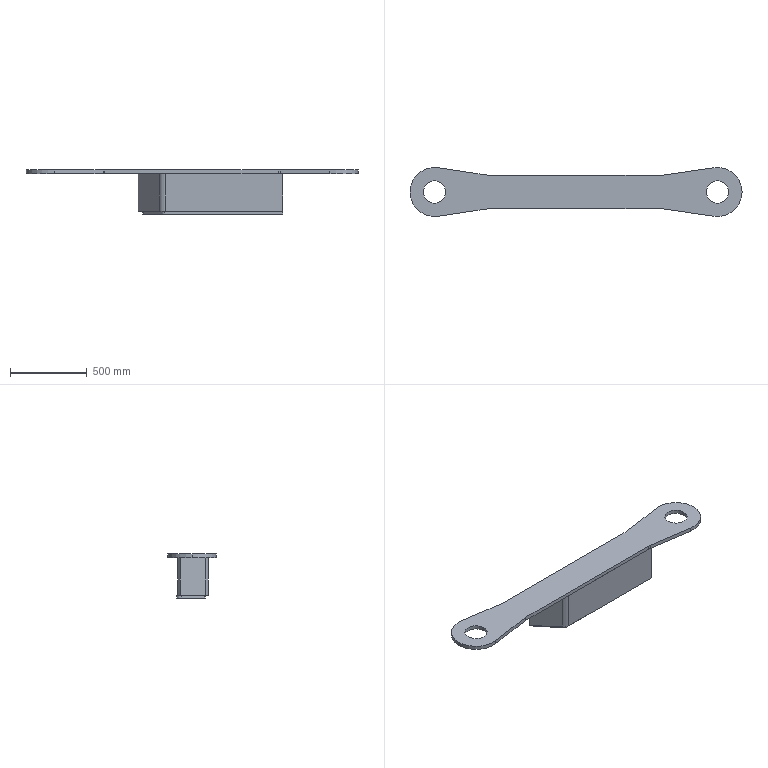Part | NX | features 后连杆左 2 | 1 solid | 48 faces | box 2165 x 320 x 288.399 mm | volume 23380345 mm3 | plane 33 | cylinder 15 | commonest cylinder face diameters 40 x4 200 x4 145 x2 320.239 x2 49.536 x1 100 x1